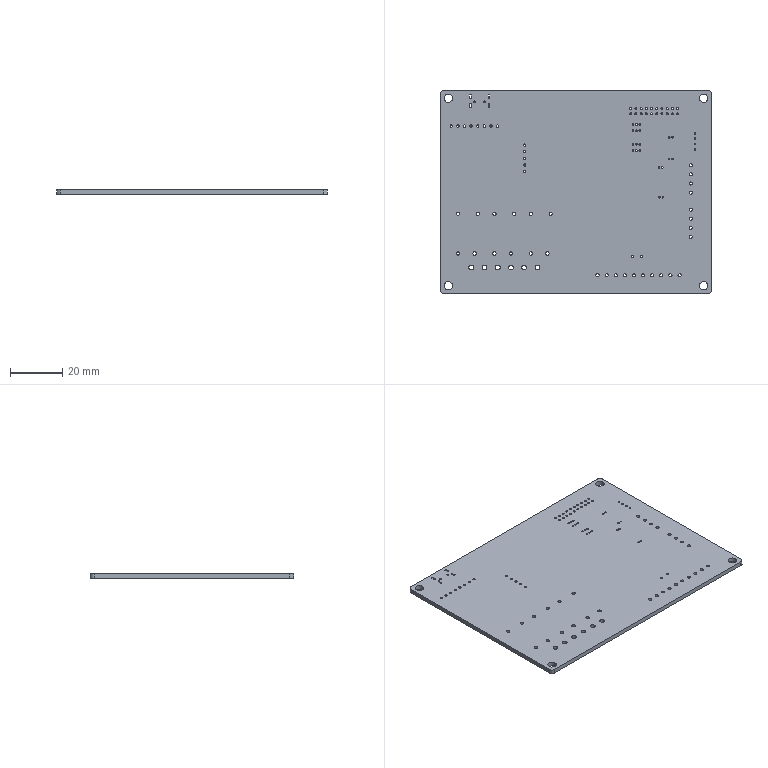Part | STEP file | RJ-USIO-V1_2-220411_307 | 1 solid | 228 faces | box 104 x 78 x 1.691 mm | volume 13523 mm3 | cylinder 214 | plane 14 | commonest cylinder face diameters 0.635 x40 0.762 x40 1.2 x36 0.9 x26 1.3 x24 0.7 x20